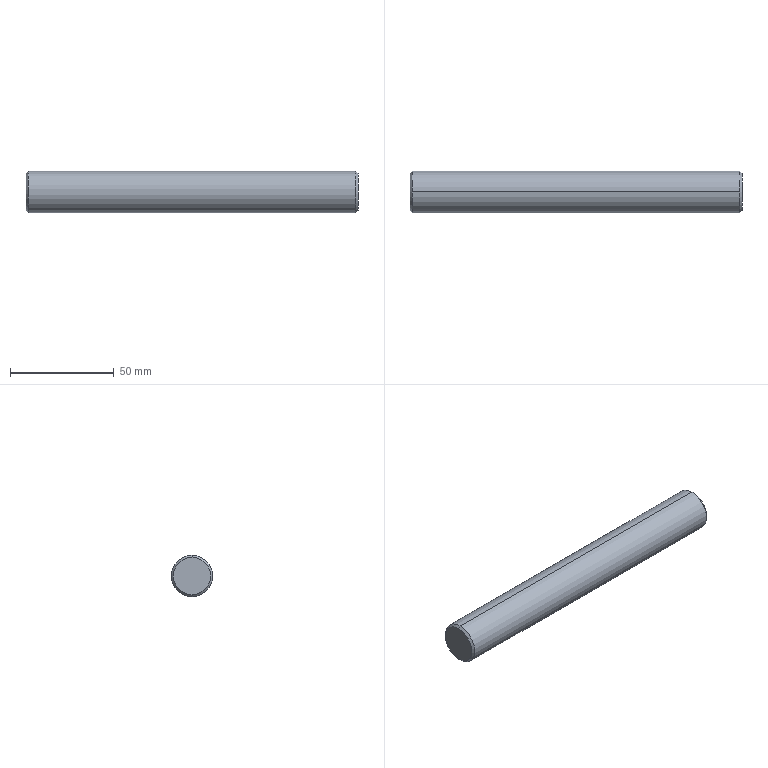Part | STEP file | 0244_005_PSSFG20-160 | 1 solid | 8 faces | box 160 x 20 x 20 mm | volume 50205 mm3 | cone 4 | cylinder 2 | plane 2 | commonest cylinder face diameters 20 x2
STEP:
#1=CARTESIAN_POINT('',(0.,0.,0.));
#2=DIRECTION('',(0.,0.,1.));
#3=DIRECTION('',(1.,0.,0.));
#4=AXIS2_PLACEMENT_3D('',#1,#2,#3);
#5=CARTESIAN_POINT('',(0.,0.,9.));
#6=VERTEX_POINT('',#5);
#7=CARTESIAN_POINT('',(0.,0.,-9.));
#8=VERTEX_POINT('',#7);
#9=CARTESIAN_POINT('',(0.,0.,0.));
#10=DIRECTION('',(-1.,0.,0.));
#11=DIRECTION('',(0.,0.,-1.));
#12=AXIS2_PLACEMENT_3D('',#9,#10,#11);
#13=CIRCLE('',#12,9.);
#14=CARTESIAN_POINT('',(0.,0.,0.));
#15=DIRECTION('',(1.,0.,0.));
#16=DIRECTION('',(0.,0.,-1.));
#17=AXIS2_PLACEMENT_3D('',#14,#15,#16);
#18=CONICAL_SURFACE('',#17,9.,0.7854);
#19=CARTESIAN_POINT('',(6.283,0.));
#20=DIRECTION('',(-1.,0.));
#21=VECTOR('',#20,1.);
#22=LINE('',#19,#21);
#23=(GEOMETRIC_REPRESENTATION_CONTEXT(2)PARAMETRIC_REPRESENTATION_CONTEXT()REPRESENTATION_CONTEXT('',''));
#24=DEFINITIONAL_REPRESENTATION('',(#22),#23);
#25=PCURVE('',#18,#24);
#26=CARTESIAN_POINT('',(0.,0.,0.));
#27=DIRECTION('',(1.,0.,0.));
#28=DIRECTION('',(0.,0.,-1.));
#29=AXIS2_PLACEMENT_3D('',#26,#27,#28);
#30=PLANE('',#29);
#31=CARTESIAN_POINT('',(9.,0.));
#32=CARTESIAN_POINT('',(9.,-15.588));
#33=CARTESIAN_POINT('',(-4.5,-7.794));
#34=CARTESIAN_POINT('',(-18.,0.));
#35=CARTESIAN_POINT('',(-4.5,7.794));
#36=CARTESIAN_POINT('',(9.,15.588));
#37=CARTESIAN_POINT('',(9.,0.));
#38=(BOUNDED_CURVE()B_SPLINE_CURVE(2,(#31,#32,#33,#34,#35,#36,#37),.UNSPECIFIED.,.T.,.F.)B_SPLINE_CURVE_WITH_KNOTS((1,2,2,2,2,1),(-2.094,0.,2.094,4.189,6.283,8.378),.UNSPECIFIED.)CURVE()GEOMETRIC_REPRESENTATION_ITEM()RATIONAL_B_SPLINE_CURVE((1.,0.5,1.,0.5,1.,0.5,1.))REPRESENTATION_ITEM(''));
#39=(GEOMETRIC_REPRESENTATION_CONTEXT(2)PARAMETRIC_REPRESENTATION_CONTEXT()REPRESENTATION_CONTEXT('',''));
#40=DEFINITIONAL_REPRESENTATION('',(#38),#39);
#41=PCURVE('',#30,#40);
#42=SURFACE_CURVE('',#13,(#25,#41),.PCURVE_S1.);
#43=EDGE_CURVE('',#6,#8,#42,.T.);
#44=ORIENTED_EDGE('',*,*,#43,.F.);
#45=CARTESIAN_POINT('',(1.,0.,10.));
#46=VERTEX_POINT('',#45);
#47=CARTESIAN_POINT('',(0.,0.,9.));
#48=DIRECTION('',(0.7071,0.,0.7071));
#49=VECTOR('',#48,1.);
#50=LINE('',#47,#49);
#51=CARTESIAN_POINT('',(3.142,0.));
#52=DIRECTION('',(0.,1.));
#53=VECTOR('',#52,1.);
#54=LINE('',#51,#53);
#55=(GEOMETRIC_REPRESENTATION_CONTEXT(2)PARAMETRIC_REPRESENTATION_CONTEXT()REPRESENTATION_CONTEXT('',''));
#56=DEFINITIONAL_REPRESENTATION('',(#54),#55);
#57=PCURVE('',#18,#56);
#58=CARTESIAN_POINT('',(0.,0.,0.));
#59=DIRECTION('',(1.,0.,0.));
#60=DIRECTION('',(0.,0.,-1.));
#61=AXIS2_PLACEMENT_3D('',#58,#59,#60);
#62=CONICAL_SURFACE('',#61,9.,0.7854);
#63=CARTESIAN_POINT('',(3.142,0.));
#64=DIRECTION('',(0.,1.));
#65=VECTOR('',#64,1.);
#66=LINE('',#63,#65);
#67=(GEOMETRIC_REPRESENTATION_CONTEXT(2)PARAMETRIC_REPRESENTATION_CONTEXT()REPRESENTATION_CONTEXT('',''));
#68=DEFINITIONAL_REPRESENTATION('',(#66),#67);
#69=PCURVE('',#62,#68);
#70=SURFACE_CURVE('',#50,(#57,#69),.PCURVE_S1.);
#71=EDGE_CURVE('',#6,#46,#70,.T.);
#72=ORIENTED_EDGE('',*,*,#71,.T.);
#73=CARTESIAN_POINT('',(1.,0.,-10.));
#74=VERTEX_POINT('',#73);
#75=CARTESIAN_POINT('',(1.,0.,0.));
#76=DIRECTION('',(1.,0.,0.));
#77=DIRECTION('',(0.,0.,-1.));
#78=AXIS2_PLACEMENT_3D('',#75,#76,#77);
#79=CIRCLE('',#78,10.);
#80=CARTESIAN_POINT('',(0.,1.));
#81=DIRECTION('',(1.,0.));
#82=VECTOR('',#81,1.);
#83=LINE('',#80,#82);
#84=(GEOMETRIC_REPRESENTATION_CONTEXT(2)PARAMETRIC_REPRESENTATION_CONTEXT()REPRESENTATION_CONTEXT('',''));
#85=DEFINITIONAL_REPRESENTATION('',(#83),#84);
#86=PCURVE('',#18,#85);
#87=CARTESIAN_POINT('',(160.,0.,0.));
#88=DIRECTION('',(-1.,0.,0.));
#89=DIRECTION('',(0.,0.,1.));
#90=AXIS2_PLACEMENT_3D('',#87,#88,#89);
#91=CYLINDRICAL_SURFACE('',#90,10.);
#92=CARTESIAN_POINT('',(3.142,159.));
#93=DIRECTION('',(-1.,0.));
#94=VECTOR('',#93,1.);
#95=LINE('',#92,#94);
#96=(GEOMETRIC_REPRESENTATION_CONTEXT(2)PARAMETRIC_REPRESENTATION_CONTEXT()REPRESENTATION_CONTEXT('',''));
#97=DEFINITIONAL_REPRESENTATION('',(#95),#96);
#98=PCURVE('',#91,#97);
#99=SURFACE_CURVE('',#79,(#86,#98),.PCURVE_S1.);
#100=EDGE_CURVE('',#74,#46,#99,.T.);
#101=ORIENTED_EDGE('',*,*,#100,.F.);
#102=CARTESIAN_POINT('',(0.,0.,-9.));
#103=DIRECTION('',(0.7071,0.,-0.7071));
#104=VECTOR('',#103,1.);
#105=LINE('',#102,#104);
#106=CARTESIAN_POINT('',(0.,0.));
#107=DIRECTION('',(0.,1.));
#108=VECTOR('',#107,1.);
#109=LINE('',#106,#108);
#110=(GEOMETRIC_REPRESENTATION_CONTEXT(2)PARAMETRIC_REPRESENTATION_CONTEXT()REPRESENTATION_CONTEXT('',''));
#111=DEFINITIONAL_REPRESENTATION('',(#109),#110);
#112=PCURVE('',#18,#111);
#113=CARTESIAN_POINT('',(6.283,0.));
#114=DIRECTION('',(0.,1.));
#115=VECTOR('',#114,1.);
#116=LINE('',#113,#115);
#117=(GEOMETRIC_REPRESENTATION_CONTEXT(2)PARAMETRIC_REPRESENTATION_CONTEXT()REPRESENTATION_CONTEXT('',''));
#118=DEFINITIONAL_REPRESENTATION('',(#116),#117);
#119=PCURVE('',#62,#118);
#120=SURFACE_CURVE('',#105,(#112,#119),.PCURVE_S1.);
#121=EDGE_CURVE('',#8,#74,#120,.T.);
#122=ORIENTED_EDGE('',*,*,#121,.F.);
#123=EDGE_LOOP('',(#44,#72,#101,#122));
#124=FACE_BOUND('',#123,.T.);
#125=ADVANCED_FACE('',(#124),#18,.T.);
#126=CARTESIAN_POINT('',(160.,0.,-9.));
#127=VERTEX_POINT('',#126);
#128=CARTESIAN_POINT('',(160.,0.,9.));
#129=VERTEX_POINT('',#128);
#130=CARTESIAN_POINT('',(160.,0.,0.));
#131=DIRECTION('',(1.,0.,0.));
#132=DIRECTION('',(0.,0.,1.));
#133=AXIS2_PLACEMENT_3D('',#130,#131,#132);
#134=CIRCLE('',#133,9.);
#135=CARTESIAN_POINT('',(159.,0.,0.));
#136=DIRECTION('',(-1.,0.,0.));
#137=DIRECTION('',(0.,0.,1.));
#138=AXIS2_PLACEMENT_3D('',#135,#136,#137);
#139=CONICAL_SURFACE('',#138,10.,0.7854);
#140=CARTESIAN_POINT('',(6.283,-1.));
#141=DIRECTION('',(-1.,0.));
#142=VECTOR('',#141,1.);
#143=LINE('',#140,#142);
#144=(GEOMETRIC_REPRESENTATION_CONTEXT(2)PARAMETRIC_REPRESENTATION_CONTEXT()REPRESENTATION_CONTEXT('',''));
#145=DEFINITIONAL_REPRESENTATION('',(#143),#144);
#146=PCURVE('',#139,#145);
#147=CARTESIAN_POINT('',(160.,10.,0.));
#148=DIRECTION('',(-1.,0.,0.));
#149=DIRECTION('',(0.,0.,1.));
#150=AXIS2_PLACEMENT_3D('',#147,#148,#149);
#151=PLANE('',#150);
#152=CARTESIAN_POINT('',(9.,-10.));
#153=CARTESIAN_POINT('',(9.,-25.588));
#154=CARTESIAN_POINT('',(-4.5,-17.794));
#155=CARTESIAN_POINT('',(-18.,-10.));
#156=CARTESIAN_POINT('',(-4.5,-2.206));
#157=CARTESIAN_POINT('',(9.,5.588));
#158=CARTESIAN_POINT('',(9.,-10.));
#159=(BOUNDED_CURVE()B_SPLINE_CURVE(2,(#152,#153,#154,#155,#156,#157,#158),.UNSPECIFIED.,.T.,.F.)B_SPLINE_CURVE_WITH_KNOTS((1,2,2,2,2,1),(-2.094,0.,2.094,4.189,6.283,8.378),.UNSPECIFIED.)CURVE()GEOMETRIC_REPRESENTATION_ITEM()RATIONAL_B_SPLINE_CURVE((1.,0.5,1.,0.5,1.,0.5,1.))REPRESENTATION_ITEM(''));
#160=(GEOMETRIC_REPRESENTATION_CONTEXT(2)PARAMETRIC_REPRESENTATION_CONTEXT()REPRESENTATION_CONTEXT('',''));
#161=DEFINITIONAL_REPRESENTATION('',(#159),#160);
#162=PCURVE('',#151,#161);
#163=SURFACE_CURVE('',#134,(#146,#162),.PCURVE_S1.);
#164=EDGE_CURVE('',#127,#129,#163,.T.);
#165=ORIENTED_EDGE('',*,*,#164,.F.);
#166=CARTESIAN_POINT('',(159.,0.,-10.));
#167=VERTEX_POINT('',#166);
#168=CARTESIAN_POINT('',(159.,0.,-10.));
#169=DIRECTION('',(-0.7071,0.,-0.7071));
#170=VECTOR('',#169,1.);
#171=LINE('',#168,#170);
#172=CARTESIAN_POINT('',(3.142,0.));
#173=DIRECTION('',(0.,1.));
#174=VECTOR('',#173,1.);
#175=LINE('',#172,#174);
#176=(GEOMETRIC_REPRESENTATION_CONTEXT(2)PARAMETRIC_REPRESENTATION_CONTEXT()REPRESENTATION_CONTEXT('',''));
#177=DEFINITIONAL_REPRESENTATION('',(#175),#176);
#178=PCURVE('',#139,#177);
#179=CARTESIAN_POINT('',(159.,0.,0.));
#180=DIRECTION('',(-1.,0.,0.));
#181=DIRECTION('',(0.,0.,1.));
#182=AXIS2_PLACEMENT_3D('',#179,#180,#181);
#183=CONICAL_SURFACE('',#182,10.,0.7854);
#184=CARTESIAN_POINT('',(3.142,0.));
#185=DIRECTION('',(0.,1.));
#186=VECTOR('',#185,1.);
#187=LINE('',#184,#186);
#188=(GEOMETRIC_REPRESENTATION_CONTEXT(2)PARAMETRIC_REPRESENTATION_CONTEXT()REPRESENTATION_CONTEXT('',''));
#189=DEFINITIONAL_REPRESENTATION('',(#187),#188);
#190=PCURVE('',#183,#189);
#191=SURFACE_CURVE('',#171,(#178,#190),.PCURVE_S1.);
#192=EDGE_CURVE('',#127,#167,#191,.T.);
#193=ORIENTED_EDGE('',*,*,#192,.T.);
#194=CARTESIAN_POINT('',(159.,0.,10.));
#195=VERTEX_POINT('',#194);
#196=CARTESIAN_POINT('',(159.,0.,0.));
#197=DIRECTION('',(-1.,0.,0.));
#198=DIRECTION('',(0.,0.,1.));
#199=AXIS2_PLACEMENT_3D('',#196,#197,#198);
#200=CIRCLE('',#199,10.);
#201=CARTESIAN_POINT('',(0.,0.));
#202=DIRECTION('',(1.,0.));
#203=VECTOR('',#202,1.);
#204=LINE('',#201,#203);
#205=(GEOMETRIC_REPRESENTATION_CONTEXT(2)PARAMETRIC_REPRESENTATION_CONTEXT()REPRESENTATION_CONTEXT('',''));
#206=DEFINITIONAL_REPRESENTATION('',(#204),#205);
#207=PCURVE('',#139,#206);
#208=CARTESIAN_POINT('',(0.,1.));
#209=DIRECTION('',(1.,0.));
#210=VECTOR('',#209,1.);
#211=LINE('',#208,#210);
#212=(GEOMETRIC_REPRESENTATION_CONTEXT(2)PARAMETRIC_REPRESENTATION_CONTEXT()REPRESENTATION_CONTEXT('',''));
#213=DEFINITIONAL_REPRESENTATION('',(#211),#212);
#214=PCURVE('',#91,#213);
#215=SURFACE_CURVE('',#200,(#207,#214),.PCURVE_S1.);
#216=EDGE_CURVE('',#195,#167,#215,.T.);
#217=ORIENTED_EDGE('',*,*,#216,.F.);
#218=CARTESIAN_POINT('',(159.,0.,10.));
#219=DIRECTION('',(-0.7071,0.,0.7071));
#220=VECTOR('',#219,1.);
#221=LINE('',#218,#220);
#222=CARTESIAN_POINT('',(0.,0.));
#223=DIRECTION('',(0.,1.));
#224=VECTOR('',#223,1.);
#225=LINE('',#222,#224);
#226=(GEOMETRIC_REPRESENTATION_CONTEXT(2)PARAMETRIC_REPRESENTATION_CONTEXT()REPRESENTATION_CONTEXT('',''));
#227=DEFINITIONAL_REPRESENTATION('',(#225),#226);
#228=PCURVE('',#139,#227);
#229=CARTESIAN_POINT('',(6.283,0.));
#230=DIRECTION('',(0.,1.));
#231=VECTOR('',#230,1.);
#232=LINE('',#229,#231);
#233=(GEOMETRIC_REPRESENTATION_CONTEXT(2)PARAMETRIC_REPRESENTATION_CONTEXT()REPRESENTATION_CONTEXT('',''));
#234=DEFINITIONAL_REPRESENTATION('',(#232),#233);
#235=PCURVE('',#183,#234);
#236=SURFACE_CURVE('',#221,(#228,#235),.PCURVE_S1.);
#237=EDGE_CURVE('',#129,#195,#236,.T.);
#238=ORIENTED_EDGE('',*,*,#237,.F.);
#239=EDGE_LOOP('',(#165,#193,#217,#238));
#240=FACE_BOUND('',#239,.T.);
#241=ADVANCED_FACE('',(#240),#139,.T.);
#242=ORIENTED_EDGE('',*,*,#216,.T.);
#243=CARTESIAN_POINT('',(160.,0.,-10.));
#244=DIRECTION('',(-1.,0.,0.));
#245=VECTOR('',#244,1.);
#246=LINE('',#243,#245);
#247=CARTESIAN_POINT('',(3.142,0.));
#248=DIRECTION('',(0.,1.));
#249=VECTOR('',#248,1.);
#250=LINE('',#247,#249);
#251=(GEOMETRIC_REPRESENTATION_CONTEXT(2)PARAMETRIC_REPRESENTATION_CONTEXT()REPRESENTATION_CONTEXT('',''));
#252=DEFINITIONAL_REPRESENTATION('',(#250),#251);
#253=PCURVE('',#91,#252);
#254=CARTESIAN_POINT('',(160.,0.,0.));
#255=DIRECTION('',(-1.,0.,0.));
#256=DIRECTION('',(0.,0.,1.));
#257=AXIS2_PLACEMENT_3D('',#254,#255,#256);
#258=CYLINDRICAL_SURFACE('',#257,10.);
#259=CARTESIAN_POINT('',(3.142,0.));
#260=DIRECTION('',(0.,1.));
#261=VECTOR('',#260,1.);
#262=LINE('',#259,#261);
#263=(GEOMETRIC_REPRESENTATION_CONTEXT(2)PARAMETRIC_REPRESENTATION_CONTEXT()REPRESENTATION_CONTEXT('',''));
#264=DEFINITIONAL_REPRESENTATION('',(#262),#263);
#265=PCURVE('',#258,#264);
#266=SURFACE_CURVE('',#246,(#253,#265),.PCURVE_S1.);
#267=EDGE_CURVE('',#167,#74,#266,.T.);
#268=ORIENTED_EDGE('',*,*,#267,.T.);
#269=ORIENTED_EDGE('',*,*,#100,.T.);
#270=CARTESIAN_POINT('',(160.,0.,10.));
#271=DIRECTION('',(-1.,0.,0.));
#272=VECTOR('',#271,1.);
#273=LINE('',#270,#272);
#274=CARTESIAN_POINT('',(0.,0.));
#275=DIRECTION('',(0.,1.));
#276=VECTOR('',#275,1.);
#277=LINE('',#274,#276);
#278=(GEOMETRIC_REPRESENTATION_CONTEXT(2)PARAMETRIC_REPRESENTATION_CONTEXT()REPRESENTATION_CONTEXT('',''));
#279=DEFINITIONAL_REPRESENTATION('',(#277),#278);
#280=PCURVE('',#91,#279);
#281=CARTESIAN_POINT('',(6.283,0.));
#282=DIRECTION('',(0.,1.));
#283=VECTOR('',#282,1.);
#284=LINE('',#281,#283);
#285=(GEOMETRIC_REPRESENTATION_CONTEXT(2)PARAMETRIC_REPRESENTATION_CONTEXT()REPRESENTATION_CONTEXT('',''));
#286=DEFINITIONAL_REPRESENTATION('',(#284),#285);
#287=PCURVE('',#258,#286);
#288=SURFACE_CURVE('',#273,(#280,#287),.PCURVE_S1.);
#289=EDGE_CURVE('',#195,#46,#288,.T.);
#290=ORIENTED_EDGE('',*,*,#289,.F.);
#291=EDGE_LOOP('',(#242,#268,#269,#290));
#292=FACE_BOUND('',#291,.T.);
#293=ADVANCED_FACE('',(#292),#91,.T.);
#294=CARTESIAN_POINT('',(0.,0.,0.));
#295=DIRECTION('',(-1.,0.,0.));
#296=DIRECTION('',(0.,0.,-1.));
#297=AXIS2_PLACEMENT_3D('',#294,#295,#296);
#298=CIRCLE('',#297,9.);
#299=CARTESIAN_POINT('',(9.,0.));
#300=CARTESIAN_POINT('',(9.,-15.588));
#301=CARTESIAN_POINT('',(-4.5,-7.794));
#302=CARTESIAN_POINT('',(-18.,0.));
#303=CARTESIAN_POINT('',(-4.5,7.794));
#304=CARTESIAN_POINT('',(9.,15.588));
#305=CARTESIAN_POINT('',(9.,0.));
#306=(BOUNDED_CURVE()B_SPLINE_CURVE(2,(#299,#300,#301,#302,#303,#304,#305),.UNSPECIFIED.,.T.,.F.)B_SPLINE_CURVE_WITH_KNOTS((1,2,2,2,2,1),(-2.094,0.,2.094,4.189,6.283,8.378),.UNSPECIFIED.)CURVE()GEOMETRIC_REPRESENTATION_ITEM()RATIONAL_B_SPLINE_CURVE((1.,0.5,1.,0.5,1.,0.5,1.))REPRESENTATION_ITEM(''));
#307=(GEOMETRIC_REPRESENTATION_CONTEXT(2)PARAMETRIC_REPRESENTATION_CONTEXT()REPRESENTATION_CONTEXT('',''));
#308=DEFINITIONAL_REPRESENTATION('',(#306),#307);
#309=PCURVE('',#30,#308);
#310=CARTESIAN_POINT('',(6.283,0.));
#311=DIRECTION('',(-1.,0.));
#312=VECTOR('',#311,1.);
#313=LINE('',#310,#312);
#314=(GEOMETRIC_REPRESENTATION_CONTEXT(2)PARAMETRIC_REPRESENTATION_CONTEXT()REPRESENTATION_CONTEXT('',''));
#315=DEFINITIONAL_REPRESENTATION('',(#313),#314);
#316=PCURVE('',#62,#315);
#317=SURFACE_CURVE('',#298,(#309,#316),.PCURVE_S1.);
#318=EDGE_CURVE('',#8,#6,#317,.T.);
#319=ORIENTED_EDGE('',*,*,#318,.T.);
#320=ORIENTED_EDGE('',*,*,#43,.T.);
#321=EDGE_LOOP('',(#319,#320));
#322=FACE_BOUND('',#321,.T.);
#323=ADVANCED_FACE('',(#322),#30,.F.);
#324=ORIENTED_EDGE('',*,*,#267,.F.);
#325=CARTESIAN_POINT('',(159.,0.,0.));
#326=DIRECTION('',(-1.,0.,0.));
#327=DIRECTION('',(0.,0.,1.));
#328=AXIS2_PLACEMENT_3D('',#325,#326,#327);
#329=CIRCLE('',#328,10.);
#330=CARTESIAN_POINT('',(0.,1.));
#331=DIRECTION('',(1.,0.));
#332=VECTOR('',#331,1.);
#333=LINE('',#330,#332);
#334=(GEOMETRIC_REPRESENTATION_CONTEXT(2)PARAMETRIC_REPRESENTATION_CONTEXT()REPRESENTATION_CONTEXT('',''));
#335=DEFINITIONAL_REPRESENTATION('',(#333),#334);
#336=PCURVE('',#258,#335);
#337=CARTESIAN_POINT('',(0.,0.));
#338=DIRECTION('',(1.,0.));
#339=VECTOR('',#338,1.);
#340=LINE('',#337,#339);
#341=(GEOMETRIC_REPRESENTATION_CONTEXT(2)PARAMETRIC_REPRESENTATION_CONTEXT()REPRESENTATION_CONTEXT('',''));
#342=DEFINITIONAL_REPRESENTATION('',(#340),#341);
#343=PCURVE('',#183,#342);
#344=SURFACE_CURVE('',#329,(#336,#343),.PCURVE_S1.);
#345=EDGE_CURVE('',#167,#195,#344,.T.);
#346=ORIENTED_EDGE('',*,*,#345,.T.);
#347=ORIENTED_EDGE('',*,*,#289,.T.);
#348=CARTESIAN_POINT('',(1.,0.,0.));
#349=DIRECTION('',(1.,0.,0.));
#350=DIRECTION('',(0.,0.,-1.));
#351=AXIS2_PLACEMENT_3D('',#348,#349,#350);
#352=CIRCLE('',#351,10.);
#353=CARTESIAN_POINT('',(9.425,159.));
#354=DIRECTION('',(-1.,0.));
#355=VECTOR('',#354,1.);
#356=LINE('',#353,#355);
#357=(GEOMETRIC_REPRESENTATION_CONTEXT(2)PARAMETRIC_REPRESENTATION_CONTEXT()REPRESENTATION_CONTEXT('',''));
#358=DEFINITIONAL_REPRESENTATION('',(#356),#357);
#359=PCURVE('',#258,#358);
#360=CARTESIAN_POINT('',(0.,1.));
#361=DIRECTION('',(1.,0.));
#362=VECTOR('',#361,1.);
#363=LINE('',#360,#362);
#364=(GEOMETRIC_REPRESENTATION_CONTEXT(2)PARAMETRIC_REPRESENTATION_CONTEXT()REPRESENTATION_CONTEXT('',''));
#365=DEFINITIONAL_REPRESENTATION('',(#363),#364);
#366=PCURVE('',#62,#365);
#367=SURFACE_CURVE('',#352,(#359,#366),.PCURVE_S1.);
#368=EDGE_CURVE('',#46,#74,#367,.T.);
#369=ORIENTED_EDGE('',*,*,#368,.T.);
#370=EDGE_LOOP('',(#324,#346,#347,#369));
#371=FACE_BOUND('',#370,.T.);
#372=ADVANCED_FACE('',(#371),#258,.T.);
#373=CARTESIAN_POINT('',(160.,0.,0.));
#374=DIRECTION('',(1.,0.,0.));
#375=DIRECTION('',(0.,0.,1.));
#376=AXIS2_PLACEMENT_3D('',#373,#374,#375);
#377=CIRCLE('',#376,9.);
#378=CARTESIAN_POINT('',(9.,-10.));
#379=CARTESIAN_POINT('',(9.,-25.588));
#380=CARTESIAN_POINT('',(-4.5,-17.794));
#381=CARTESIAN_POINT('',(-18.,-10.));
#382=CARTESIAN_POINT('',(-4.5,-2.206));
#383=CARTESIAN_POINT('',(9.,5.588));
#384=CARTESIAN_POINT('',(9.,-10.));
#385=(BOUNDED_CURVE()B_SPLINE_CURVE(2,(#378,#379,#380,#381,#382,#383,#384),.UNSPECIFIED.,.T.,.F.)B_SPLINE_CURVE_WITH_KNOTS((1,2,2,2,2,1),(-2.094,0.,2.094,4.189,6.283,8.378),.UNSPECIFIED.)CURVE()GEOMETRIC_REPRESENTATION_ITEM()RATIONAL_B_SPLINE_CURVE((1.,0.5,1.,0.5,1.,0.5,1.))REPRESENTATION_ITEM(''));
#386=(GEOMETRIC_REPRESENTATION_CONTEXT(2)PARAMETRIC_REPRESENTATION_CONTEXT()REPRESENTATION_CONTEXT('',''));
#387=DEFINITIONAL_REPRESENTATION('',(#385),#386);
#388=PCURVE('',#151,#387);
#389=CARTESIAN_POINT('',(6.283,-1.));
#390=DIRECTION('',(-1.,0.));
#391=VECTOR('',#390,1.);
#392=LINE('',#389,#391);
#393=(GEOMETRIC_REPRESENTATION_CONTEXT(2)PARAMETRIC_REPRESENTATION_CONTEXT()REPRESENTATION_CONTEXT('',''));
#394=DEFINITIONAL_REPRESENTATION('',(#392),#393);
#395=PCURVE('',#183,#394);
#396=SURFACE_CURVE('',#377,(#388,#395),.PCURVE_S1.);
#397=EDGE_CURVE('',#129,#127,#396,.T.);
#398=ORIENTED_EDGE('',*,*,#397,.T.);
#399=ORIENTED_EDGE('',*,*,#164,.T.);
#400=EDGE_LOOP('',(#398,#399));
#401=FACE_BOUND('',#400,.T.);
#402=ADVANCED_FACE('',(#401),#151,.F.);
#403=ORIENTED_EDGE('',*,*,#192,.F.);
#404=ORIENTED_EDGE('',*,*,#397,.F.);
#405=ORIENTED_EDGE('',*,*,#237,.T.);
#406=ORIENTED_EDGE('',*,*,#345,.F.);
#407=EDGE_LOOP('',(#403,#404,#405,#406));
#408=FACE_BOUND('',#407,.T.);
#409=ADVANCED_FACE('',(#408),#183,.T.);
#410=ORIENTED_EDGE('',*,*,#71,.F.);
#411=ORIENTED_EDGE('',*,*,#318,.F.);
#412=ORIENTED_EDGE('',*,*,#121,.T.);
#413=ORIENTED_EDGE('',*,*,#368,.F.);
#414=EDGE_LOOP('',(#410,#411,#412,#413));
#415=FACE_BOUND('',#414,.T.);
#416=ADVANCED_FACE('',(#415),#62,.T.);
#417=CLOSED_SHELL('',(#125,#241,#293,#323,#372,#402,#409,#416));
#418=MANIFOLD_SOLID_BREP('',#417);
#419=(LENGTH_UNIT()NAMED_UNIT(*)SI_UNIT(.MILLI.,.METRE.));
#420=UNCERTAINTY_MEASURE_WITH_UNIT(LENGTH_MEASURE(0.0000001),#419,'','');
#421=(NAMED_UNIT(*)PLANE_ANGLE_UNIT()SI_UNIT($,.RADIAN.));
#422=(NAMED_UNIT(*)SI_UNIT($,.STERADIAN.)SOLID_ANGLE_UNIT());
#423=(GEOMETRIC_REPRESENTATION_CONTEXT(3)GLOBAL_UNCERTAINTY_ASSIGNED_CONTEXT((#420))GLOBAL_UNIT_ASSIGNED_CONTEXT((#419,#421,#422))REPRESENTATION_CONTEXT('',''));
#424=ADVANCED_BREP_SHAPE_REPRESENTATION('',(#4,#418),#423);